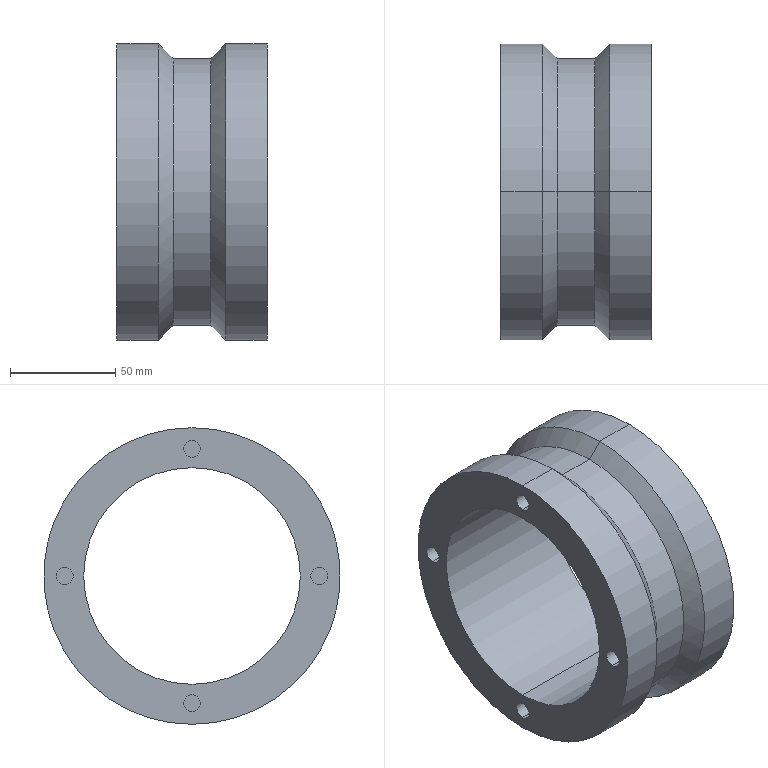Part | SolidWorks | features ICE 2, Revolution 1 | 1 solid | 38 faces | box 71.5 x 141 x 141 mm | volume 441421 mm3 | cylinder 24 | plane 10 | cone 4 | commonest cylinder face diameters 8 x16 141 x4 103 x2 127 x2
STEP:
#1=CARTESIAN_POINT('',(21.275,0.,64.5));
#2=VERTEX_POINT('',#1);
#3=CARTESIAN_POINT('',(21.275,0.,56.5));
#4=VERTEX_POINT('',#3);
#5=CARTESIAN_POINT('',(21.275,0.,60.5));
#6=DIRECTION('',(1.,0.,0.));
#7=DIRECTION('',(0.,0.,-1.));
#8=AXIS2_PLACEMENT_3D('',#5,#6,#7);
#9=CIRCLE('',#8,4.);
#10=EDGE_CURVE('',#2,#4,#9,.T.);
#11=ORIENTED_EDGE('',*,*,#10,.F.);
#12=CARTESIAN_POINT('',(34.275,0.,64.5));
#13=VERTEX_POINT('',#12);
#14=CARTESIAN_POINT('',(21.275,0.,64.5));
#15=DIRECTION('',(1.,0.,0.));
#16=VECTOR('',#15,1000.);
#17=LINE('',#14,#16);
#18=EDGE_CURVE('',#2,#13,#17,.T.);
#19=ORIENTED_EDGE('',*,*,#18,.T.);
#20=CARTESIAN_POINT('',(34.275,0.,56.5));
#21=VERTEX_POINT('',#20);
#22=CARTESIAN_POINT('',(34.275,0.,60.5));
#23=DIRECTION('',(1.,0.,0.));
#24=DIRECTION('',(0.,0.,-1.));
#25=AXIS2_PLACEMENT_3D('',#22,#23,#24);
#26=CIRCLE('',#25,4.);
#27=EDGE_CURVE('',#13,#21,#26,.T.);
#28=ORIENTED_EDGE('',*,*,#27,.T.);
#29=CARTESIAN_POINT('',(21.275,0.,56.5));
#30=DIRECTION('',(1.,0.,0.));
#31=VECTOR('',#30,1000.);
#32=LINE('',#29,#31);
#33=EDGE_CURVE('',#4,#21,#32,.T.);
#34=ORIENTED_EDGE('',*,*,#33,.F.);
#35=EDGE_LOOP('',(#11,#19,#28,#34));
#36=FACE_OUTER_BOUND('',#35,.T.);
#37=CARTESIAN_POINT('',(21.275,0.,60.5));
#38=DIRECTION('',(1.,0.,0.));
#39=DIRECTION('',(0.,0.,-1.));
#40=AXIS2_PLACEMENT_3D('',#37,#38,#39);
#41=CYLINDRICAL_SURFACE('',#40,4.);
#42=ADVANCED_FACE('',(#36),#41,.F.);
#43=CARTESIAN_POINT('',(21.275,60.5,4.));
#44=VERTEX_POINT('',#43);
#45=CARTESIAN_POINT('',(21.275,60.5,-4.));
#46=VERTEX_POINT('',#45);
#47=CARTESIAN_POINT('',(21.275,60.5,0.));
#48=DIRECTION('',(1.,0.,0.));
#49=DIRECTION('',(0.,0.,-1.));
#50=AXIS2_PLACEMENT_3D('',#47,#48,#49);
#51=CIRCLE('',#50,4.);
#52=EDGE_CURVE('',#44,#46,#51,.T.);
#53=ORIENTED_EDGE('',*,*,#52,.F.);
#54=CARTESIAN_POINT('',(34.275,60.5,4.));
#55=VERTEX_POINT('',#54);
#56=CARTESIAN_POINT('',(21.275,60.5,4.));
#57=DIRECTION('',(1.,0.,0.));
#58=VECTOR('',#57,1000.);
#59=LINE('',#56,#58);
#60=EDGE_CURVE('',#44,#55,#59,.T.);
#61=ORIENTED_EDGE('',*,*,#60,.T.);
#62=CARTESIAN_POINT('',(34.275,60.5,-4.));
#63=VERTEX_POINT('',#62);
#64=CARTESIAN_POINT('',(34.275,60.5,0.));
#65=DIRECTION('',(1.,0.,0.));
#66=DIRECTION('',(0.,0.,-1.));
#67=AXIS2_PLACEMENT_3D('',#64,#65,#66);
#68=CIRCLE('',#67,4.);
#69=EDGE_CURVE('',#55,#63,#68,.T.);
#70=ORIENTED_EDGE('',*,*,#69,.T.);
#71=CARTESIAN_POINT('',(21.275,60.5,-4.));
#72=DIRECTION('',(1.,0.,0.));
#73=VECTOR('',#72,1000.);
#74=LINE('',#71,#73);
#75=EDGE_CURVE('',#46,#63,#74,.T.);
#76=ORIENTED_EDGE('',*,*,#75,.F.);
#77=EDGE_LOOP('',(#53,#61,#70,#76));
#78=FACE_OUTER_BOUND('',#77,.T.);
#79=CARTESIAN_POINT('',(21.275,60.5,0.));
#80=DIRECTION('',(1.,0.,0.));
#81=DIRECTION('',(0.,0.,-1.));
#82=AXIS2_PLACEMENT_3D('',#79,#80,#81);
#83=CYLINDRICAL_SURFACE('',#82,4.);
#84=ADVANCED_FACE('',(#78),#83,.F.);
#85=CARTESIAN_POINT('',(21.275,0.,-56.5));
#86=VERTEX_POINT('',#85);
#87=CARTESIAN_POINT('',(21.275,0.,-64.5));
#88=VERTEX_POINT('',#87);
#89=CARTESIAN_POINT('',(21.275,0.,-60.5));
#90=DIRECTION('',(1.,0.,0.));
#91=DIRECTION('',(0.,0.,-1.));
#92=AXIS2_PLACEMENT_3D('',#89,#90,#91);
#93=CIRCLE('',#92,4.);
#94=EDGE_CURVE('',#86,#88,#93,.T.);
#95=ORIENTED_EDGE('',*,*,#94,.F.);
#96=CARTESIAN_POINT('',(34.275,0.,-56.5));
#97=VERTEX_POINT('',#96);
#98=CARTESIAN_POINT('',(21.275,0.,-56.5));
#99=DIRECTION('',(1.,0.,0.));
#100=VECTOR('',#99,1000.);
#101=LINE('',#98,#100);
#102=EDGE_CURVE('',#86,#97,#101,.T.);
#103=ORIENTED_EDGE('',*,*,#102,.T.);
#104=CARTESIAN_POINT('',(34.275,0.,-64.5));
#105=VERTEX_POINT('',#104);
#106=CARTESIAN_POINT('',(34.275,0.,-60.5));
#107=DIRECTION('',(1.,0.,0.));
#108=DIRECTION('',(0.,0.,-1.));
#109=AXIS2_PLACEMENT_3D('',#106,#107,#108);
#110=CIRCLE('',#109,4.);
#111=EDGE_CURVE('',#97,#105,#110,.T.);
#112=ORIENTED_EDGE('',*,*,#111,.T.);
#113=CARTESIAN_POINT('',(21.275,0.,-64.5));
#114=DIRECTION('',(1.,0.,0.));
#115=VECTOR('',#114,1000.);
#116=LINE('',#113,#115);
#117=EDGE_CURVE('',#88,#105,#116,.T.);
#118=ORIENTED_EDGE('',*,*,#117,.F.);
#119=EDGE_LOOP('',(#95,#103,#112,#118));
#120=FACE_OUTER_BOUND('',#119,.T.);
#121=CARTESIAN_POINT('',(21.275,0.,-60.5));
#122=DIRECTION('',(1.,0.,0.));
#123=DIRECTION('',(0.,0.,-1.));
#124=AXIS2_PLACEMENT_3D('',#121,#122,#123);
#125=CYLINDRICAL_SURFACE('',#124,4.);
#126=ADVANCED_FACE('',(#120),#125,.F.);
#127=CARTESIAN_POINT('',(21.275,-60.5,4.));
#128=VERTEX_POINT('',#127);
#129=CARTESIAN_POINT('',(21.275,-60.5,-4.));
#130=VERTEX_POINT('',#129);
#131=CARTESIAN_POINT('',(21.275,-60.5,0.));
#132=DIRECTION('',(1.,0.,0.));
#133=DIRECTION('',(0.,0.,-1.));
#134=AXIS2_PLACEMENT_3D('',#131,#132,#133);
#135=CIRCLE('',#134,4.);
#136=EDGE_CURVE('',#128,#130,#135,.T.);
#137=ORIENTED_EDGE('',*,*,#136,.F.);
#138=CARTESIAN_POINT('',(34.275,-60.5,4.));
#139=VERTEX_POINT('',#138);
#140=CARTESIAN_POINT('',(21.275,-60.5,4.));
#141=DIRECTION('',(1.,0.,0.));
#142=VECTOR('',#141,1000.);
#143=LINE('',#140,#142);
#144=EDGE_CURVE('',#128,#139,#143,.T.);
#145=ORIENTED_EDGE('',*,*,#144,.T.);
#146=CARTESIAN_POINT('',(34.275,-60.5,-4.));
#147=VERTEX_POINT('',#146);
#148=CARTESIAN_POINT('',(34.275,-60.5,0.));
#149=DIRECTION('',(1.,0.,0.));
#150=DIRECTION('',(0.,0.,-1.));
#151=AXIS2_PLACEMENT_3D('',#148,#149,#150);
#152=CIRCLE('',#151,4.);
#153=EDGE_CURVE('',#139,#147,#152,.T.);
#154=ORIENTED_EDGE('',*,*,#153,.T.);
#155=CARTESIAN_POINT('',(21.275,-60.5,-4.));
#156=DIRECTION('',(1.,0.,0.));
#157=VECTOR('',#156,1000.);
#158=LINE('',#155,#157);
#159=EDGE_CURVE('',#130,#147,#158,.T.);
#160=ORIENTED_EDGE('',*,*,#159,.F.);
#161=EDGE_LOOP('',(#137,#145,#154,#160));
#162=FACE_OUTER_BOUND('',#161,.T.);
#163=CARTESIAN_POINT('',(21.275,-60.5,0.));
#164=DIRECTION('',(1.,0.,0.));
#165=DIRECTION('',(0.,0.,-1.));
#166=AXIS2_PLACEMENT_3D('',#163,#164,#165);
#167=CYLINDRICAL_SURFACE('',#166,4.);
#168=ADVANCED_FACE('',(#162),#167,.F.);
#169=CARTESIAN_POINT('',(-24.225,0.,-64.5));
#170=VERTEX_POINT('',#169);
#171=CARTESIAN_POINT('',(-24.225,0.,-56.5));
#172=VERTEX_POINT('',#171);
#173=CARTESIAN_POINT('',(-24.225,0.,-60.5));
#174=DIRECTION('',(-1.,0.,0.));
#175=DIRECTION('',(0.,0.,1.));
#176=AXIS2_PLACEMENT_3D('',#173,#174,#175);
#177=CIRCLE('',#176,4.);
#178=EDGE_CURVE('',#170,#172,#177,.T.);
#179=ORIENTED_EDGE('',*,*,#178,.F.);
#180=CARTESIAN_POINT('',(-37.225,0.,-64.5));
#181=VERTEX_POINT('',#180);
#182=CARTESIAN_POINT('',(-24.225,0.,-64.5));
#183=DIRECTION('',(-1.,0.,0.));
#184=VECTOR('',#183,1000.);
#185=LINE('',#182,#184);
#186=EDGE_CURVE('',#170,#181,#185,.T.);
#187=ORIENTED_EDGE('',*,*,#186,.T.);
#188=CARTESIAN_POINT('',(-37.225,0.,-56.5));
#189=VERTEX_POINT('',#188);
#190=CARTESIAN_POINT('',(-37.225,0.,-60.5));
#191=DIRECTION('',(-1.,0.,0.));
#192=DIRECTION('',(0.,0.,1.));
#193=AXIS2_PLACEMENT_3D('',#190,#191,#192);
#194=CIRCLE('',#193,4.);
#195=EDGE_CURVE('',#181,#189,#194,.T.);
#196=ORIENTED_EDGE('',*,*,#195,.T.);
#197=CARTESIAN_POINT('',(-24.225,0.,-56.5));
#198=DIRECTION('',(-1.,0.,0.));
#199=VECTOR('',#198,1000.);
#200=LINE('',#197,#199);
#201=EDGE_CURVE('',#172,#189,#200,.T.);
#202=ORIENTED_EDGE('',*,*,#201,.F.);
#203=EDGE_LOOP('',(#179,#187,#196,#202));
#204=FACE_OUTER_BOUND('',#203,.T.);
#205=CARTESIAN_POINT('',(-24.225,0.,-60.5));
#206=DIRECTION('',(-1.,0.,0.));
#207=DIRECTION('',(0.,0.,1.));
#208=AXIS2_PLACEMENT_3D('',#205,#206,#207);
#209=CYLINDRICAL_SURFACE('',#208,4.);
#210=ADVANCED_FACE('',(#204),#209,.F.);
#211=CARTESIAN_POINT('',(-24.225,60.5,-4.));
#212=VERTEX_POINT('',#211);
#213=CARTESIAN_POINT('',(-24.225,60.5,4.));
#214=VERTEX_POINT('',#213);
#215=CARTESIAN_POINT('',(-24.225,60.5,0.));
#216=DIRECTION('',(-1.,0.,0.));
#217=DIRECTION('',(0.,0.,1.));
#218=AXIS2_PLACEMENT_3D('',#215,#216,#217);
#219=CIRCLE('',#218,4.);
#220=EDGE_CURVE('',#212,#214,#219,.T.);
#221=ORIENTED_EDGE('',*,*,#220,.F.);
#222=CARTESIAN_POINT('',(-37.225,60.5,-4.));
#223=VERTEX_POINT('',#222);
#224=CARTESIAN_POINT('',(-24.225,60.5,-4.));
#225=DIRECTION('',(-1.,0.,0.));
#226=VECTOR('',#225,1000.);
#227=LINE('',#224,#226);
#228=EDGE_CURVE('',#212,#223,#227,.T.);
#229=ORIENTED_EDGE('',*,*,#228,.T.);
#230=CARTESIAN_POINT('',(-37.225,60.5,4.));
#231=VERTEX_POINT('',#230);
#232=CARTESIAN_POINT('',(-37.225,60.5,0.));
#233=DIRECTION('',(-1.,0.,0.));
#234=DIRECTION('',(0.,0.,1.));
#235=AXIS2_PLACEMENT_3D('',#232,#233,#234);
#236=CIRCLE('',#235,4.);
#237=EDGE_CURVE('',#223,#231,#236,.T.);
#238=ORIENTED_EDGE('',*,*,#237,.T.);
#239=CARTESIAN_POINT('',(-24.225,60.5,4.));
#240=DIRECTION('',(-1.,0.,0.));
#241=VECTOR('',#240,1000.);
#242=LINE('',#239,#241);
#243=EDGE_CURVE('',#214,#231,#242,.T.);
#244=ORIENTED_EDGE('',*,*,#243,.F.);
#245=EDGE_LOOP('',(#221,#229,#238,#244));
#246=FACE_OUTER_BOUND('',#245,.T.);
#247=CARTESIAN_POINT('',(-24.225,60.5,0.));
#248=DIRECTION('',(-1.,0.,0.));
#249=DIRECTION('',(0.,0.,1.));
#250=AXIS2_PLACEMENT_3D('',#247,#248,#249);
#251=CYLINDRICAL_SURFACE('',#250,4.);
#252=ADVANCED_FACE('',(#246),#251,.F.);
#253=CARTESIAN_POINT('',(-24.225,0.,56.5));
#254=VERTEX_POINT('',#253);
#255=CARTESIAN_POINT('',(-24.225,0.,64.5));
#256=VERTEX_POINT('',#255);
#257=CARTESIAN_POINT('',(-24.225,0.,60.5));
#258=DIRECTION('',(-1.,0.,0.));
#259=DIRECTION('',(0.,0.,1.));
#260=AXIS2_PLACEMENT_3D('',#257,#258,#259);
#261=CIRCLE('',#260,4.);
#262=EDGE_CURVE('',#254,#256,#261,.T.);
#263=ORIENTED_EDGE('',*,*,#262,.F.);
#264=CARTESIAN_POINT('',(-37.225,0.,56.5));
#265=VERTEX_POINT('',#264);
#266=CARTESIAN_POINT('',(-24.225,0.,56.5));
#267=DIRECTION('',(-1.,0.,0.));
#268=VECTOR('',#267,1000.);
#269=LINE('',#266,#268);
#270=EDGE_CURVE('',#254,#265,#269,.T.);
#271=ORIENTED_EDGE('',*,*,#270,.T.);
#272=CARTESIAN_POINT('',(-37.225,0.,64.5));
#273=VERTEX_POINT('',#272);
#274=CARTESIAN_POINT('',(-37.225,0.,60.5));
#275=DIRECTION('',(-1.,0.,0.));
#276=DIRECTION('',(0.,0.,1.));
#277=AXIS2_PLACEMENT_3D('',#274,#275,#276);
#278=CIRCLE('',#277,4.);
#279=EDGE_CURVE('',#265,#273,#278,.T.);
#280=ORIENTED_EDGE('',*,*,#279,.T.);
#281=CARTESIAN_POINT('',(-24.225,0.,64.5));
#282=DIRECTION('',(-1.,0.,0.));
#283=VECTOR('',#282,1000.);
#284=LINE('',#281,#283);
#285=EDGE_CURVE('',#256,#273,#284,.T.);
#286=ORIENTED_EDGE('',*,*,#285,.F.);
#287=EDGE_LOOP('',(#263,#271,#280,#286));
#288=FACE_OUTER_BOUND('',#287,.T.);
#289=CARTESIAN_POINT('',(-24.225,0.,60.5));
#290=DIRECTION('',(-1.,0.,0.));
#291=DIRECTION('',(0.,0.,1.));
#292=AXIS2_PLACEMENT_3D('',#289,#290,#291);
#293=CYLINDRICAL_SURFACE('',#292,4.);
#294=ADVANCED_FACE('',(#288),#293,.F.);
#295=CARTESIAN_POINT('',(-24.225,-60.5,-4.));
#296=VERTEX_POINT('',#295);
#297=CARTESIAN_POINT('',(-24.225,-60.5,4.));
#298=VERTEX_POINT('',#297);
#299=CARTESIAN_POINT('',(-24.225,-60.5,0.));
#300=DIRECTION('',(-1.,0.,0.));
#301=DIRECTION('',(0.,0.,1.));
#302=AXIS2_PLACEMENT_3D('',#299,#300,#301);
#303=CIRCLE('',#302,4.);
#304=EDGE_CURVE('',#296,#298,#303,.T.);
#305=ORIENTED_EDGE('',*,*,#304,.F.);
#306=CARTESIAN_POINT('',(-37.225,-60.5,-4.));
#307=VERTEX_POINT('',#306);
#308=CARTESIAN_POINT('',(-24.225,-60.5,-4.));
#309=DIRECTION('',(-1.,0.,0.));
#310=VECTOR('',#309,1000.);
#311=LINE('',#308,#310);
#312=EDGE_CURVE('',#296,#307,#311,.T.);
#313=ORIENTED_EDGE('',*,*,#312,.T.);
#314=CARTESIAN_POINT('',(-37.225,-60.5,4.));
#315=VERTEX_POINT('',#314);
#316=CARTESIAN_POINT('',(-37.225,-60.5,0.));
#317=DIRECTION('',(-1.,0.,0.));
#318=DIRECTION('',(0.,0.,1.));
#319=AXIS2_PLACEMENT_3D('',#316,#317,#318);
#320=CIRCLE('',#319,4.);
#321=EDGE_CURVE('',#307,#315,#320,.T.);
#322=ORIENTED_EDGE('',*,*,#321,.T.);
#323=CARTESIAN_POINT('',(-24.225,-60.5,4.));
#324=DIRECTION('',(-1.,0.,0.));
#325=VECTOR('',#324,1000.);
#326=LINE('',#323,#325);
#327=EDGE_CURVE('',#298,#315,#326,.T.);
#328=ORIENTED_EDGE('',*,*,#327,.F.);
#329=EDGE_LOOP('',(#305,#313,#322,#328));
#330=FACE_OUTER_BOUND('',#329,.T.);
#331=CARTESIAN_POINT('',(-24.225,-60.5,0.));
#332=DIRECTION('',(-1.,0.,0.));
#333=DIRECTION('',(0.,0.,1.));
#334=AXIS2_PLACEMENT_3D('',#331,#332,#333);
#335=CYLINDRICAL_SURFACE('',#334,4.);
#336=ADVANCED_FACE('',(#330),#335,.F.);
#337=CARTESIAN_POINT('',(-10.475,0.,63.5));
#338=VERTEX_POINT('',#337);
#339=CARTESIAN_POINT('',(-10.475,0.,-63.5));
#340=VERTEX_POINT('',#339);
#341=CARTESIAN_POINT('',(-10.475,0.,0.));
#342=DIRECTION('',(-1.,0.,0.));
#343=DIRECTION('',(0.,0.,1.));
#344=AXIS2_PLACEMENT_3D('',#341,#342,#343);
#345=CIRCLE('',#344,63.5);
#346=EDGE_CURVE('',#338,#340,#345,.T.);
#347=ORIENTED_EDGE('',*,*,#346,.T.);
#348=CARTESIAN_POINT('',(-17.475,0.,-70.5));
#349=VERTEX_POINT('',#348);
#350=CARTESIAN_POINT('',(-10.475,0.,-63.5));
#351=DIRECTION('',(-0.7071,0.,-0.7071));
#352=VECTOR('',#351,1000.);
#353=LINE('',#350,#352);
#354=EDGE_CURVE('',#340,#349,#353,.T.);
#355=ORIENTED_EDGE('',*,*,#354,.T.);
#356=CARTESIAN_POINT('',(-17.475,0.,70.5));
#357=VERTEX_POINT('',#356);
#358=CARTESIAN_POINT('',(-17.475,0.,0.));
#359=DIRECTION('',(-1.,0.,0.));
#360=DIRECTION('',(0.,0.,1.));
#361=AXIS2_PLACEMENT_3D('',#358,#359,#360);
#362=CIRCLE('',#361,70.5);
#363=EDGE_CURVE('',#357,#349,#362,.T.);
#364=ORIENTED_EDGE('',*,*,#363,.F.);
#365=CARTESIAN_POINT('',(-10.475,0.,63.5));
#366=DIRECTION('',(-0.7071,0.,0.7071));
#367=VECTOR('',#366,1000.);
#368=LINE('',#365,#367);
#369=EDGE_CURVE('',#338,#357,#368,.T.);
#370=ORIENTED_EDGE('',*,*,#369,.F.);
#371=EDGE_LOOP('',(#347,#355,#364,#370));
#372=FACE_OUTER_BOUND('',#371,.T.);
#373=CARTESIAN_POINT('',(-10.475,0.,0.));
#374=DIRECTION('',(-1.,0.,0.));
#375=DIRECTION('',(0.,0.,1.));
#376=AXIS2_PLACEMENT_3D('',#373,#374,#375);
#377=CONICAL_SURFACE('',#376,63.5,0.7854);
#378=ADVANCED_FACE('',(#372),#377,.T.);
#379=CARTESIAN_POINT('',(7.525,0.,63.5));
#380=VERTEX_POINT('',#379);
#381=CARTESIAN_POINT('',(7.525,0.,-63.5));
#382=VERTEX_POINT('',#381);
#383=CARTESIAN_POINT('',(7.525,0.,0.));
#384=DIRECTION('',(-1.,0.,0.));
#385=DIRECTION('',(0.,0.,1.));
#386=AXIS2_PLACEMENT_3D('',#383,#384,#385);
#387=CIRCLE('',#386,63.5);
#388=EDGE_CURVE('',#380,#382,#387,.T.);
#389=ORIENTED_EDGE('',*,*,#388,.T.);
#390=CARTESIAN_POINT('',(-86.708,0.,-63.5));
#391=DIRECTION('',(-1.,0.,0.));
#392=VECTOR('',#391,1000.);
#393=LINE('',#390,#392);
#394=EDGE_CURVE('',#382,#340,#393,.T.);
#395=ORIENTED_EDGE('',*,*,#394,.T.);
#396=ORIENTED_EDGE('',*,*,#346,.F.);
#397=CARTESIAN_POINT('',(-86.708,0.,63.5));
#398=DIRECTION('',(-1.,0.,0.));
#399=VECTOR('',#398,1000.);
#400=LINE('',#397,#399);
#401=EDGE_CURVE('',#380,#338,#400,.T.);
#402=ORIENTED_EDGE('',*,*,#401,.F.);
#403=EDGE_LOOP('',(#389,#395,#396,#402));
#404=FACE_OUTER_BOUND('',#403,.T.);
#405=CARTESIAN_POINT('',(-86.708,0.,0.));
#406=DIRECTION('',(-1.,0.,0.));
#407=DIRECTION('',(0.,0.,1.));
#408=AXIS2_PLACEMENT_3D('',#405,#406,#407);
#409=CYLINDRICAL_SURFACE('',#408,63.5);
#410=ADVANCED_FACE('',(#404),#409,.T.);
#411=ORIENTED_EDGE('',*,*,#388,.F.);
#412=CARTESIAN_POINT('',(14.525,0.,70.5));
#413=VERTEX_POINT('',#412);
#414=CARTESIAN_POINT('',(14.525,0.,70.5));
#415=DIRECTION('',(0.7071,0.,0.7071));
#416=VECTOR('',#415,1000.);
#417=LINE('',#414,#416);
#418=EDGE_CURVE('',#380,#413,#417,.T.);
#419=ORIENTED_EDGE('',*,*,#418,.T.);
#420=CARTESIAN_POINT('',(14.525,0.,-70.5));
#421=VERTEX_POINT('',#420);
#422=CARTESIAN_POINT('',(14.525,0.,0.));
#423=DIRECTION('',(-1.,0.,0.));
#424=DIRECTION('',(0.,0.,1.));
#425=AXIS2_PLACEMENT_3D('',#422,#423,#424);
#426=CIRCLE('',#425,70.5);
#427=EDGE_CURVE('',#413,#421,#426,.T.);
#428=ORIENTED_EDGE('',*,*,#427,.T.);
#429=CARTESIAN_POINT('',(14.525,0.,-70.5));
#430=DIRECTION('',(0.7071,0.,-0.7071));
#431=VECTOR('',#430,1000.);
#432=LINE('',#429,#431);
#433=EDGE_CURVE('',#382,#421,#432,.T.);
#434=ORIENTED_EDGE('',*,*,#433,.F.);
#435=EDGE_LOOP('',(#411,#419,#428,#434));
#436=FACE_OUTER_BOUND('',#435,.T.);
#437=CARTESIAN_POINT('',(14.525,0.,0.));
#438=DIRECTION('',(1.,0.,0.));
#439=DIRECTION('',(0.,0.,-1.));
#440=AXIS2_PLACEMENT_3D('',#437,#438,#439);
#441=CONICAL_SURFACE('',#440,70.5,0.7854);
#442=ADVANCED_FACE('',(#436),#441,.T.);
#443=CARTESIAN_POINT('',(34.275,0.,70.5));
#444=VERTEX_POINT('',#443);
#445=CARTESIAN_POINT('',(34.275,0.,-70.5));
#446=VERTEX_POINT('',#445);
#447=CARTESIAN_POINT('',(34.275,0.,0.));
#448=DIRECTION('',(-1.,0.,0.));
#449=DIRECTION('',(0.,0.,1.));
#450=AXIS2_PLACEMENT_3D('',#447,#448,#449);
#451=CIRCLE('',#450,70.5);
#452=EDGE_CURVE('',#444,#446,#451,.T.);
#453=ORIENTED_EDGE('',*,*,#452,.T.);
#454=CARTESIAN_POINT('',(-86.708,0.,-70.5));
#455=DIRECTION('',(-1.,0.,0.));
#456=VECTOR('',#455,1000.);
#457=LINE('',#454,#456);
#458=EDGE_CURVE('',#446,#421,#457,.T.);
#459=ORIENTED_EDGE('',*,*,#458,.T.);
#460=ORIENTED_EDGE('',*,*,#427,.F.);
#461=CARTESIAN_POINT('',(-86.708,0.,70.5));
#462=DIRECTION('',(-1.,0.,0.));
#463=VECTOR('',#462,1000.);
#464=LINE('',#461,#463);
#465=EDGE_CURVE('',#444,#413,#464,.T.);
#466=ORIENTED_EDGE('',*,*,#465,.F.);
#467=EDGE_LOOP('',(#453,#459,#460,#466));
#468=FACE_OUTER_BOUND('',#467,.T.);
#469=CARTESIAN_POINT('',(-86.708,0.,0.));
#470=DIRECTION('',(-1.,0.,0.));
#471=DIRECTION('',(0.,0.,1.));
#472=AXIS2_PLACEMENT_3D('',#469,#470,#471);
#473=CYLINDRICAL_SURFACE('',#472,70.5);
#474=ADVANCED_FACE('',(#468),#473,.T.);
#475=CARTESIAN_POINT('',(34.275,0.,-51.5));
#476=VERTEX_POINT('',#475);
#477=CARTESIAN_POINT('',(34.275,0.,51.5));
#478=VERTEX_POINT('',#477);
#479=CARTESIAN_POINT('',(34.275,0.,0.));
#480=DIRECTION('',(-1.,0.,0.));
#481=DIRECTION('',(0.,0.,1.));
#482=AXIS2_PLACEMENT_3D('',#479,#480,#481);
#483=CIRCLE('',#482,51.5);
#484=EDGE_CURVE('',#476,#478,#483,.T.);
#485=ORIENTED_EDGE('',*,*,#484,.F.);
#486=CARTESIAN_POINT('',(-37.225,0.,-51.5));
#487=VERTEX_POINT('',#486);
#488=CARTESIAN_POINT('',(-86.708,0.,-51.5));
#489=DIRECTION('',(-1.,0.,0.));
#490=VECTOR('',#489,1000.);
#491=LINE('',#488,#490);
#492=EDGE_CURVE('',#476,#487,#491,.T.);
#493=ORIENTED_EDGE('',*,*,#492,.T.);
#494=CARTESIAN_POINT('',(-37.225,0.,51.5));
#495=VERTEX_POINT('',#494);
#496=CARTESIAN_POINT('',(-37.225,0.,0.));
#497=DIRECTION('',(-1.,0.,0.));
#498=DIRECTION('',(0.,0.,1.));
#499=AXIS2_PLACEMENT_3D('',#496,#497,#498);
#500=CIRCLE('',#499,51.5);
#501=EDGE_CURVE('',#487,#495,#500,.T.);
#502=ORIENTED_EDGE('',*,*,#501,.T.);
#503=CARTESIAN_POINT('',(-86.708,0.,51.5));
#504=DIRECTION('',(-1.,0.,0.));
#505=VECTOR('',#504,1000.);
#506=LINE('',#503,#505);
#507=EDGE_CURVE('',#478,#495,#506,.T.);
#508=ORIENTED_EDGE('',*,*,#507,.F.);
#509=EDGE_LOOP('',(#485,#493,#502,#508));
#510=FACE_OUTER_BOUND('',#509,.T.);
#511=CARTESIAN_POINT('',(-86.708,0.,0.));
#512=DIRECTION('',(-1.,0.,0.));
#513=DIRECTION('',(0.,0.,1.));
#514=AXIS2_PLACEMENT_3D('',#511,#512,#513);
#515=CYLINDRICAL_SURFACE('',#514,51.5);
#516=ADVANCED_FACE('',(#510),#515,.F.);
#517=ORIENTED_EDGE('',*,*,#363,.T.);
#518=CARTESIAN_POINT('',(-37.225,0.,-70.5));
#519=VERTEX_POINT('',#518);
#520=CARTESIAN_POINT('',(-86.708,0.,-70.5));
#521=DIRECTION('',(-1.,0.,0.));
#522=VECTOR('',#521,1000.);
#523=LINE('',#520,#522);
#524=EDGE_CURVE('',#349,#519,#523,.T.);
#525=ORIENTED_EDGE('',*,*,#524,.T.);
#526=CARTESIAN_POINT('',(-37.225,0.,70.5));
#527=VERTEX_POINT('',#526);
#528=CARTESIAN_POINT('',(-37.225,0.,0.));
#529=DIRECTION('',(-1.,0.,0.));
#530=DIRECTION('',(0.,0.,1.));
#531=AXIS2_PLACEMENT_3D('',#528,#529,#530);
#532=CIRCLE('',#531,70.5);
#533=EDGE_CURVE('',#527,#519,#532,.T.);
#534=ORIENTED_EDGE('',*,*,#533,.F.);
#535=CARTESIAN_POINT('',(-86.708,0.,70.5));
#536=DIRECTION('',(-1.,0.,0.));
#537=VECTOR('',#536,1000.);
#538=LINE('',#535,#537);
#539=EDGE_CURVE('',#357,#527,#538,.T.);
#540=ORIENTED_EDGE('',*,*,#539,.F.);
#541=EDGE_LOOP('',(#517,#525,#534,#540));
#542=FACE_OUTER_BOUND('',#541,.T.);
#543=CARTESIAN_POINT('',(-86.708,0.,0.));
#544=DIRECTION('',(-1.,0.,0.));
#545=DIRECTION('',(0.,0.,1.));
#546=AXIS2_PLACEMENT_3D('',#543,#544,#545);
#547=CYLINDRICAL_SURFACE('',#546,70.5);
#548=ADVANCED_FACE('',(#542),#547,.T.);
#549=ORIENTED_EDGE('',*,*,#524,.F.);
#550=CARTESIAN_POINT('',(-17.475,0.,0.));
#551=DIRECTION('',(-1.,0.,0.));
#552=DIRECTION('',(0.,0.,1.));
#553=AXIS2_PLACEMENT_3D('',#550,#551,#552);
#554=CIRCLE('',#553,70.5);
#555=EDGE_CURVE('',#349,#357,#554,.T.);
#556=ORIENTED_EDGE('',*,*,#555,.T.);
#557=ORIENTED_EDGE('',*,*,#539,.T.);
#558=CARTESIAN_POINT('',(-37.225,0.,0.));
#559=DIRECTION('',(-1.,0.,0.));
#560=DIRECTION('',(0.,0.,1.));
#561=AXIS2_PLACEMENT_3D('',#558,#559,#560);
#562=CIRCLE('',#561,70.5);
#563=EDGE_CURVE('',#519,#527,#562,.T.);
#564=ORIENTED_EDGE('',*,*,#563,.F.);
#565=EDGE_LOOP('',(#549,#556,#557,#564));
#566=FACE_OUTER_BOUND('',#565,.T.);
#567=CARTESIAN_POINT('',(-86.708,0.,0.));
#568=DIRECTION('',(-1.,0.,0.));
#569=DIRECTION('',(0.,0.,1.));
#570=AXIS2_PLACEMENT_3D('',#567,#568,#569);
#571=CYLINDRICAL_SURFACE('',#570,70.5);
#572=ADVANCED_FACE('',(#566),#571,.T.);
#573=CARTESIAN_POINT('',(-37.225,0.,-60.5));
#574=DIRECTION('',(-1.,0.,0.));
#575=DIRECTION('',(0.,0.,1.));
#576=AXIS2_PLACEMENT_3D('',#573,#574,#575);
#577=CIRCLE('',#576,4.);
#578=EDGE_CURVE('',#189,#181,#577,.T.);
#579=ORIENTED_EDGE('',*,*,#578,.F.);
#580=ORIENTED_EDGE('',*,*,#195,.F.);
#581=EDGE_LOOP('',(#579,#580));
#582=FACE_BOUND('',#581,.T.);
#583=CARTESIAN_POINT('',(-37.225,60.5,0.));
#584=DIRECTION('',(-1.,0.,0.));
#585=DIRECTION('',(0.,0.,1.));
#586=AXIS2_PLACEMENT_3D('',#583,#584,#585);
#587=CIRCLE('',#586,4.);
#588=EDGE_CURVE('',#231,#223,#587,.T.);
#589=ORIENTED_EDGE('',*,*,#588,.F.);
#590=ORIENTED_EDGE('',*,*,#237,.F.);
#591=EDGE_LOOP('',(#589,#590));
#592=FACE_BOUND('',#591,.T.);
#593=CARTESIAN_POINT('',(-37.225,0.,60.5));
#594=DIRECTION('',(-1.,0.,0.));
#595=DIRECTION('',(0.,0.,1.));
#596=AXIS2_PLACEMENT_3D('',#593,#594,#595);
#597=CIRCLE('',#596,4.);
#598=EDGE_CURVE('',#273,#265,#597,.T.);
#599=ORIENTED_EDGE('',*,*,#598,.F.);
#600=ORIENTED_EDGE('',*,*,#279,.F.);
#601=EDGE_LOOP('',(#599,#600));
#602=FACE_BOUND('',#601,.T.);
#603=CARTESIAN_POINT('',(-37.225,-60.5,0.));
#604=DIRECTION('',(-1.,0.,0.));
#605=DIRECTION('',(0.,0.,1.));
#606=AXIS2_PLACEMENT_3D('',#603,#604,#605);
#607=CIRCLE('',#606,4.);
#608=EDGE_CURVE('',#315,#307,#607,.T.);
#609=ORIENTED_EDGE('',*,*,#608,.F.);
#610=ORIENTED_EDGE('',*,*,#321,.F.);
#611=EDGE_LOOP('',(#609,#610));
#612=FACE_BOUND('',#611,.T.);
#613=CARTESIAN_POINT('',(-37.225,0.,0.));
#614=DIRECTION('',(-1.,0.,0.));
#615=DIRECTION('',(0.,0.,1.));
#616=AXIS2_PLACEMENT_3D('',#613,#614,#615);
#617=CIRCLE('',#616,51.5);
#618=EDGE_CURVE('',#495,#487,#617,.T.);
#619=ORIENTED_EDGE('',*,*,#618,.F.);
#620=ORIENTED_EDGE('',*,*,#501,.F.);
#621=EDGE_LOOP('',(#619,#620));
#622=FACE_BOUND('',#621,.T.);
#623=ORIENTED_EDGE('',*,*,#533,.T.);
#624=ORIENTED_EDGE('',*,*,#563,.T.);
#625=EDGE_LOOP('',(#623,#624));
#626=FACE_OUTER_BOUND('',#625,.T.);
#627=CARTESIAN_POINT('',(-37.225,70.5,0.));
#628=DIRECTION('',(1.,0.,0.));
#629=DIRECTION('',(0.,0.,-1.));
#630=AXIS2_PLACEMENT_3D('',#627,#628,#629);
#631=PLANE('',#630);
#632=ADVANCED_FACE('',(#582,#592,#602,#612,#622,#626),#631,.F.);
#633=ORIENTED_EDGE('',*,*,#492,.F.);
#634=CARTESIAN_POINT('',(34.275,0.,0.));
#635=DIRECTION('',(-1.,0.,0.));
#636=DIRECTION('',(0.,0.,1.));
#637=AXIS2_PLACEMENT_3D('',#634,#635,#636);
#638=CIRCLE('',#637,51.5);
#639=EDGE_CURVE('',#478,#476,#638,.T.);
#640=ORIENTED_EDGE('',*,*,#639,.F.);
#641=ORIENTED_EDGE('',*,*,#507,.T.);
#642=ORIENTED_EDGE('',*,*,#618,.T.);
#643=EDGE_LOOP('',(#633,#640,#641,#642));
#644=FACE_OUTER_BOUND('',#643,.T.);
#645=CARTESIAN_POINT('',(-86.708,0.,0.));
#646=DIRECTION('',(-1.,0.,0.));
#647=DIRECTION('',(0.,0.,1.));
#648=AXIS2_PLACEMENT_3D('',#645,#646,#647);
#649=CYLINDRICAL_SURFACE('',#648,51.5);
#650=ADVANCED_FACE('',(#644),#649,.F.);
#651=CARTESIAN_POINT('',(34.275,0.,60.5));
#652=DIRECTION('',(1.,0.,0.));
#653=DIRECTION('',(0.,0.,-1.));
#654=AXIS2_PLACEMENT_3D('',#651,#652,#653);
#655=CIRCLE('',#654,4.);
#656=EDGE_CURVE('',#21,#13,#655,.T.);
#657=ORIENTED_EDGE('',*,*,#656,.F.);
#658=ORIENTED_EDGE('',*,*,#27,.F.);
#659=EDGE_LOOP('',(#657,#658));
#660=FACE_BOUND('',#659,.T.);
#661=CARTESIAN_POINT('',(34.275,60.5,0.));
#662=DIRECTION('',(1.,0.,0.));
#663=DIRECTION('',(0.,0.,-1.));
#664=AXIS2_PLACEMENT_3D('',#661,#662,#663);
#665=CIRCLE('',#664,4.);
#666=EDGE_CURVE('',#63,#55,#665,.T.);
#667=ORIENTED_EDGE('',*,*,#666,.F.);
#668=ORIENTED_EDGE('',*,*,#69,.F.);
#669=EDGE_LOOP('',(#667,#668));
#670=FACE_BOUND('',#669,.T.);
#671=CARTESIAN_POINT('',(34.275,0.,-60.5));
#672=DIRECTION('',(1.,0.,0.));
#673=DIRECTION('',(0.,0.,-1.));
#674=AXIS2_PLACEMENT_3D('',#671,#672,#673);
#675=CIRCLE('',#674,4.);
#676=EDGE_CURVE('',#105,#97,#675,.T.);
#677=ORIENTED_EDGE('',*,*,#676,.F.);
#678=ORIENTED_EDGE('',*,*,#111,.F.);
#679=EDGE_LOOP('',(#677,#678));
#680=FACE_BOUND('',#679,.T.);
#681=CARTESIAN_POINT('',(34.275,-60.5,0.));
#682=DIRECTION('',(1.,0.,0.));
#683=DIRECTION('',(0.,0.,-1.));
#684=AXIS2_PLACEMENT_3D('',#681,#682,#683);
#685=CIRCLE('',#684,4.);
#686=EDGE_CURVE('',#147,#139,#685,.T.);
#687=ORIENTED_EDGE('',*,*,#686,.F.);
#688=ORIENTED_EDGE('',*,*,#153,.F.);
#689=EDGE_LOOP('',(#687,#688));
#690=FACE_BOUND('',#689,.T.);
#691=ORIENTED_EDGE('',*,*,#452,.F.);
#692=CARTESIAN_POINT('',(34.275,0.,0.));
#693=DIRECTION('',(-1.,0.,0.));
#694=DIRECTION('',(0.,0.,1.));
#695=AXIS2_PLACEMENT_3D('',#692,#693,#694);
#696=CIRCLE('',#695,70.5);
#697=EDGE_CURVE('',#446,#444,#696,.T.);
#698=ORIENTED_EDGE('',*,*,#697,.F.);
#699=EDGE_LOOP('',(#691,#698));
#700=FACE_OUTER_BOUND('',#699,.T.);
#701=ORIENTED_EDGE('',*,*,#639,.T.);
#702=ORIENTED_EDGE('',*,*,#484,.T.);
#703=EDGE_LOOP('',(#701,#702));
#704=FACE_BOUND('',#703,.T.);
#705=CARTESIAN_POINT('',(34.275,51.5,0.));
#706=DIRECTION('',(-1.,0.,0.));
#707=DIRECTION('',(0.,0.,1.));
#708=AXIS2_PLACEMENT_3D('',#705,#706,#707);
#709=PLANE('',#708);
#710=ADVANCED_FACE('',(#660,#670,#680,#690,#700,#704),#709,.F.);
#711=ORIENTED_EDGE('',*,*,#458,.F.);
#712=ORIENTED_EDGE('',*,*,#697,.T.);
#713=ORIENTED_EDGE('',*,*,#465,.T.);
#714=CARTESIAN_POINT('',(14.525,0.,0.));
#715=DIRECTION('',(-1.,0.,0.));
#716=DIRECTION('',(0.,0.,1.));
#717=AXIS2_PLACEMENT_3D('',#714,#715,#716);
#718=CIRCLE('',#717,70.5);
#719=EDGE_CURVE('',#421,#413,#718,.T.);
#720=ORIENTED_EDGE('',*,*,#719,.F.);
#721=EDGE_LOOP('',(#711,#712,#713,#720));
#722=FACE_OUTER_BOUND('',#721,.T.);
#723=CARTESIAN_POINT('',(-86.708,0.,0.));
#724=DIRECTION('',(-1.,0.,0.));
#725=DIRECTION('',(0.,0.,1.));
#726=AXIS2_PLACEMENT_3D('',#723,#724,#725);
#727=CYLINDRICAL_SURFACE('',#726,70.5);
#728=ADVANCED_FACE('',(#722),#727,.T.);
#729=ORIENTED_EDGE('',*,*,#418,.F.);
#730=CARTESIAN_POINT('',(7.525,0.,0.));
#731=DIRECTION('',(-1.,0.,0.));
#732=DIRECTION('',(0.,0.,1.));
#733=AXIS2_PLACEMENT_3D('',#730,#731,#732);
#734=CIRCLE('',#733,63.5);
#735=EDGE_CURVE('',#382,#380,#734,.T.);
#736=ORIENTED_EDGE('',*,*,#735,.F.);
#737=ORIENTED_EDGE('',*,*,#433,.T.);
#738=ORIENTED_EDGE('',*,*,#719,.T.);
#739=EDGE_LOOP('',(#729,#736,#737,#738));
#740=FACE_OUTER_BOUND('',#739,.T.);
#741=CARTESIAN_POINT('',(14.525,0.,0.));
#742=DIRECTION('',(1.,0.,0.));
#743=DIRECTION('',(0.,0.,-1.));
#744=AXIS2_PLACEMENT_3D('',#741,#742,#743);
#745=CONICAL_SURFACE('',#744,70.5,0.7854);
#746=ADVANCED_FACE('',(#740),#745,.T.);
#747=ORIENTED_EDGE('',*,*,#394,.F.);
#748=ORIENTED_EDGE('',*,*,#735,.T.);
#749=ORIENTED_EDGE('',*,*,#401,.T.);
#750=CARTESIAN_POINT('',(-10.475,0.,0.));
#751=DIRECTION('',(-1.,0.,0.));
#752=DIRECTION('',(0.,0.,1.));
#753=AXIS2_PLACEMENT_3D('',#750,#751,#752);
#754=CIRCLE('',#753,63.5);
#755=EDGE_CURVE('',#340,#338,#754,.T.);
#756=ORIENTED_EDGE('',*,*,#755,.F.);
#757=EDGE_LOOP('',(#747,#748,#749,#756));
#758=FACE_OUTER_BOUND('',#757,.T.);
#759=CARTESIAN_POINT('',(-86.708,0.,0.));
#760=DIRECTION('',(-1.,0.,0.));
#761=DIRECTION('',(0.,0.,1.));
#762=AXIS2_PLACEMENT_3D('',#759,#760,#761);
#763=CYLINDRICAL_SURFACE('',#762,63.5);
#764=ADVANCED_FACE('',(#758),#763,.T.);
#765=ORIENTED_EDGE('',*,*,#354,.F.);
#766=ORIENTED_EDGE('',*,*,#755,.T.);
#767=ORIENTED_EDGE('',*,*,#369,.T.);
#768=ORIENTED_EDGE('',*,*,#555,.F.);
#769=EDGE_LOOP('',(#765,#766,#767,#768));
#770=FACE_OUTER_BOUND('',#769,.T.);
#771=CARTESIAN_POINT('',(-10.475,0.,0.));
#772=DIRECTION('',(-1.,0.,0.));
#773=DIRECTION('',(0.,0.,1.));
#774=AXIS2_PLACEMENT_3D('',#771,#772,#773);
#775=CONICAL_SURFACE('',#774,63.5,0.7854);
#776=ADVANCED_FACE('',(#770),#775,.T.);
#777=ORIENTED_EDGE('',*,*,#312,.F.);
#778=CARTESIAN_POINT('',(-24.225,-60.5,0.));
#779=DIRECTION('',(-1.,0.,0.));
#780=DIRECTION('',(0.,0.,1.));
#781=AXIS2_PLACEMENT_3D('',#778,#779,#780);
#782=CIRCLE('',#781,4.);
#783=EDGE_CURVE('',#298,#296,#782,.T.);
#784=ORIENTED_EDGE('',*,*,#783,.F.);
#785=ORIENTED_EDGE('',*,*,#327,.T.);
#786=ORIENTED_EDGE('',*,*,#608,.T.);
#787=EDGE_LOOP('',(#777,#784,#785,#786));
#788=FACE_OUTER_BOUND('',#787,.T.);
#789=CARTESIAN_POINT('',(-24.225,-60.5,0.));
#790=DIRECTION('',(-1.,0.,0.));
#791=DIRECTION('',(0.,0.,1.));
#792=AXIS2_PLACEMENT_3D('',#789,#790,#791);
#793=CYLINDRICAL_SURFACE('',#792,4.);
#794=ADVANCED_FACE('',(#788),#793,.F.);
#795=ORIENTED_EDGE('',*,*,#783,.T.);
#796=ORIENTED_EDGE('',*,*,#304,.T.);
#797=EDGE_LOOP('',(#795,#796));
#798=FACE_OUTER_BOUND('',#797,.T.);
#799=CARTESIAN_POINT('',(-24.225,-60.5,0.));
#800=DIRECTION('',(-1.,0.,0.));
#801=DIRECTION('',(0.,0.,1.));
#802=AXIS2_PLACEMENT_3D('',#799,#800,#801);
#803=PLANE('',#802);
#804=ADVANCED_FACE('',(#798),#803,.T.);
#805=ORIENTED_EDGE('',*,*,#270,.F.);
#806=CARTESIAN_POINT('',(-24.225,0.,60.5));
#807=DIRECTION('',(-1.,0.,0.));
#808=DIRECTION('',(0.,0.,1.));
#809=AXIS2_PLACEMENT_3D('',#806,#807,#808);
#810=CIRCLE('',#809,4.);
#811=EDGE_CURVE('',#256,#254,#810,.T.);
#812=ORIENTED_EDGE('',*,*,#811,.F.);
#813=ORIENTED_EDGE('',*,*,#285,.T.);
#814=ORIENTED_EDGE('',*,*,#598,.T.);
#815=EDGE_LOOP('',(#805,#812,#813,#814));
#816=FACE_OUTER_BOUND('',#815,.T.);
#817=CARTESIAN_POINT('',(-24.225,0.,60.5));
#818=DIRECTION('',(-1.,0.,0.));
#819=DIRECTION('',(0.,0.,1.));
#820=AXIS2_PLACEMENT_3D('',#817,#818,#819);
#821=CYLINDRICAL_SURFACE('',#820,4.);
#822=ADVANCED_FACE('',(#816),#821,.F.);
#823=ORIENTED_EDGE('',*,*,#811,.T.);
#824=ORIENTED_EDGE('',*,*,#262,.T.);
#825=EDGE_LOOP('',(#823,#824));
#826=FACE_OUTER_BOUND('',#825,.T.);
#827=CARTESIAN_POINT('',(-24.225,0.,60.5));
#828=DIRECTION('',(-1.,0.,0.));
#829=DIRECTION('',(0.,0.,1.));
#830=AXIS2_PLACEMENT_3D('',#827,#828,#829);
#831=PLANE('',#830);
#832=ADVANCED_FACE('',(#826),#831,.T.);
#833=ORIENTED_EDGE('',*,*,#228,.F.);
#834=CARTESIAN_POINT('',(-24.225,60.5,0.));
#835=DIRECTION('',(-1.,0.,0.));
#836=DIRECTION('',(0.,0.,1.));
#837=AXIS2_PLACEMENT_3D('',#834,#835,#836);
#838=CIRCLE('',#837,4.);
#839=EDGE_CURVE('',#214,#212,#838,.T.);
#840=ORIENTED_EDGE('',*,*,#839,.F.);
#841=ORIENTED_EDGE('',*,*,#243,.T.);
#842=ORIENTED_EDGE('',*,*,#588,.T.);
#843=EDGE_LOOP('',(#833,#840,#841,#842));
#844=FACE_OUTER_BOUND('',#843,.T.);
#845=CARTESIAN_POINT('',(-24.225,60.5,0.));
#846=DIRECTION('',(-1.,0.,0.));
#847=DIRECTION('',(0.,0.,1.));
#848=AXIS2_PLACEMENT_3D('',#845,#846,#847);
#849=CYLINDRICAL_SURFACE('',#848,4.);
#850=ADVANCED_FACE('',(#844),#849,.F.);
#851=ORIENTED_EDGE('',*,*,#839,.T.);
#852=ORIENTED_EDGE('',*,*,#220,.T.);
#853=EDGE_LOOP('',(#851,#852));
#854=FACE_OUTER_BOUND('',#853,.T.);
#855=CARTESIAN_POINT('',(-24.225,60.5,0.));
#856=DIRECTION('',(-1.,0.,0.));
#857=DIRECTION('',(0.,0.,1.));
#858=AXIS2_PLACEMENT_3D('',#855,#856,#857);
#859=PLANE('',#858);
#860=ADVANCED_FACE('',(#854),#859,.T.);
#861=ORIENTED_EDGE('',*,*,#186,.F.);
#862=CARTESIAN_POINT('',(-24.225,0.,-60.5));
#863=DIRECTION('',(-1.,0.,0.));
#864=DIRECTION('',(0.,0.,1.));
#865=AXIS2_PLACEMENT_3D('',#862,#863,#864);
#866=CIRCLE('',#865,4.);
#867=EDGE_CURVE('',#172,#170,#866,.T.);
#868=ORIENTED_EDGE('',*,*,#867,.F.);
#869=ORIENTED_EDGE('',*,*,#201,.T.);
#870=ORIENTED_EDGE('',*,*,#578,.T.);
#871=EDGE_LOOP('',(#861,#868,#869,#870));
#872=FACE_OUTER_BOUND('',#871,.T.);
#873=CARTESIAN_POINT('',(-24.225,0.,-60.5));
#874=DIRECTION('',(-1.,0.,0.));
#875=DIRECTION('',(0.,0.,1.));
#876=AXIS2_PLACEMENT_3D('',#873,#874,#875);
#877=CYLINDRICAL_SURFACE('',#876,4.);
#878=ADVANCED_FACE('',(#872),#877,.F.);
#879=ORIENTED_EDGE('',*,*,#867,.T.);
#880=ORIENTED_EDGE('',*,*,#178,.T.);
#881=EDGE_LOOP('',(#879,#880));
#882=FACE_OUTER_BOUND('',#881,.T.);
#883=CARTESIAN_POINT('',(-24.225,0.,-60.5));
#884=DIRECTION('',(-1.,0.,0.));
#885=DIRECTION('',(0.,0.,1.));
#886=AXIS2_PLACEMENT_3D('',#883,#884,#885);
#887=PLANE('',#886);
#888=ADVANCED_FACE('',(#882),#887,.T.);
#889=ORIENTED_EDGE('',*,*,#144,.F.);
#890=CARTESIAN_POINT('',(21.275,-60.5,0.));
#891=DIRECTION('',(1.,0.,0.));
#892=DIRECTION('',(0.,0.,-1.));
#893=AXIS2_PLACEMENT_3D('',#890,#891,#892);
#894=CIRCLE('',#893,4.);
#895=EDGE_CURVE('',#130,#128,#894,.T.);
#896=ORIENTED_EDGE('',*,*,#895,.F.);
#897=ORIENTED_EDGE('',*,*,#159,.T.);
#898=ORIENTED_EDGE('',*,*,#686,.T.);
#899=EDGE_LOOP('',(#889,#896,#897,#898));
#900=FACE_OUTER_BOUND('',#899,.T.);
#901=CARTESIAN_POINT('',(21.275,-60.5,0.));
#902=DIRECTION('',(1.,0.,0.));
#903=DIRECTION('',(0.,0.,-1.));
#904=AXIS2_PLACEMENT_3D('',#901,#902,#903);
#905=CYLINDRICAL_SURFACE('',#904,4.);
#906=ADVANCED_FACE('',(#900),#905,.F.);
#907=ORIENTED_EDGE('',*,*,#895,.T.);
#908=ORIENTED_EDGE('',*,*,#136,.T.);
#909=EDGE_LOOP('',(#907,#908));
#910=FACE_OUTER_BOUND('',#909,.T.);
#911=CARTESIAN_POINT('',(21.275,-60.5,0.));
#912=DIRECTION('',(1.,0.,0.));
#913=DIRECTION('',(0.,0.,-1.));
#914=AXIS2_PLACEMENT_3D('',#911,#912,#913);
#915=PLANE('',#914);
#916=ADVANCED_FACE('',(#910),#915,.T.);
#917=ORIENTED_EDGE('',*,*,#102,.F.);
#918=CARTESIAN_POINT('',(21.275,0.,-60.5));
#919=DIRECTION('',(1.,0.,0.));
#920=DIRECTION('',(0.,0.,-1.));
#921=AXIS2_PLACEMENT_3D('',#918,#919,#920);
#922=CIRCLE('',#921,4.);
#923=EDGE_CURVE('',#88,#86,#922,.T.);
#924=ORIENTED_EDGE('',*,*,#923,.F.);
#925=ORIENTED_EDGE('',*,*,#117,.T.);
#926=ORIENTED_EDGE('',*,*,#676,.T.);
#927=EDGE_LOOP('',(#917,#924,#925,#926));
#928=FACE_OUTER_BOUND('',#927,.T.);
#929=CARTESIAN_POINT('',(21.275,0.,-60.5));
#930=DIRECTION('',(1.,0.,0.));
#931=DIRECTION('',(0.,0.,-1.));
#932=AXIS2_PLACEMENT_3D('',#929,#930,#931);
#933=CYLINDRICAL_SURFACE('',#932,4.);
#934=ADVANCED_FACE('',(#928),#933,.F.);
#935=ORIENTED_EDGE('',*,*,#923,.T.);
#936=ORIENTED_EDGE('',*,*,#94,.T.);
#937=EDGE_LOOP('',(#935,#936));
#938=FACE_OUTER_BOUND('',#937,.T.);
#939=CARTESIAN_POINT('',(21.275,0.,-60.5));
#940=DIRECTION('',(1.,0.,0.));
#941=DIRECTION('',(0.,0.,-1.));
#942=AXIS2_PLACEMENT_3D('',#939,#940,#941);
#943=PLANE('',#942);
#944=ADVANCED_FACE('',(#938),#943,.T.);
#945=ORIENTED_EDGE('',*,*,#60,.F.);
#946=CARTESIAN_POINT('',(21.275,60.5,0.));
#947=DIRECTION('',(1.,0.,0.));
#948=DIRECTION('',(0.,0.,-1.));
#949=AXIS2_PLACEMENT_3D('',#946,#947,#948);
#950=CIRCLE('',#949,4.);
#951=EDGE_CURVE('',#46,#44,#950,.T.);
#952=ORIENTED_EDGE('',*,*,#951,.F.);
#953=ORIENTED_EDGE('',*,*,#75,.T.);
#954=ORIENTED_EDGE('',*,*,#666,.T.);
#955=EDGE_LOOP('',(#945,#952,#953,#954));
#956=FACE_OUTER_BOUND('',#955,.T.);
#957=CARTESIAN_POINT('',(21.275,60.5,0.));
#958=DIRECTION('',(1.,0.,0.));
#959=DIRECTION('',(0.,0.,-1.));
#960=AXIS2_PLACEMENT_3D('',#957,#958,#959);
#961=CYLINDRICAL_SURFACE('',#960,4.);
#962=ADVANCED_FACE('',(#956),#961,.F.);
#963=ORIENTED_EDGE('',*,*,#951,.T.);
#964=ORIENTED_EDGE('',*,*,#52,.T.);
#965=EDGE_LOOP('',(#963,#964));
#966=FACE_OUTER_BOUND('',#965,.T.);
#967=CARTESIAN_POINT('',(21.275,60.5,0.));
#968=DIRECTION('',(1.,0.,0.));
#969=DIRECTION('',(0.,0.,-1.));
#970=AXIS2_PLACEMENT_3D('',#967,#968,#969);
#971=PLANE('',#970);
#972=ADVANCED_FACE('',(#966),#971,.T.);
#973=ORIENTED_EDGE('',*,*,#18,.F.);
#974=CARTESIAN_POINT('',(21.275,0.,60.5));
#975=DIRECTION('',(1.,0.,0.));
#976=DIRECTION('',(0.,0.,-1.));
#977=AXIS2_PLACEMENT_3D('',#974,#975,#976);
#978=CIRCLE('',#977,4.);
#979=EDGE_CURVE('',#4,#2,#978,.T.);
#980=ORIENTED_EDGE('',*,*,#979,.F.);
#981=ORIENTED_EDGE('',*,*,#33,.T.);
#982=ORIENTED_EDGE('',*,*,#656,.T.);
#983=EDGE_LOOP('',(#973,#980,#981,#982));
#984=FACE_OUTER_BOUND('',#983,.T.);
#985=CARTESIAN_POINT('',(21.275,0.,60.5));
#986=DIRECTION('',(1.,0.,0.));
#987=DIRECTION('',(0.,0.,-1.));
#988=AXIS2_PLACEMENT_3D('',#985,#986,#987);
#989=CYLINDRICAL_SURFACE('',#988,4.);
#990=ADVANCED_FACE('',(#984),#989,.F.);
#991=ORIENTED_EDGE('',*,*,#979,.T.);
#992=ORIENTED_EDGE('',*,*,#10,.T.);
#993=EDGE_LOOP('',(#991,#992));
#994=FACE_OUTER_BOUND('',#993,.T.);
#995=CARTESIAN_POINT('',(21.275,0.,60.5));
#996=DIRECTION('',(1.,0.,0.));
#997=DIRECTION('',(0.,0.,-1.));
#998=AXIS2_PLACEMENT_3D('',#995,#996,#997);
#999=PLANE('',#998);
#1000=ADVANCED_FACE('',(#994),#999,.T.);
#1001=CLOSED_SHELL('',(#42,#84,#126,#168,#210,#252,#294,#336,#378,#410,#442,#474,#516,#548,#572,#632,#650,#710,#728,#746,#764,#776,#794,#804,#822,#832,#850,#860,#878,#888,#906,#916,#934,#944,#962,#972,#990,#1000));
#1002=MANIFOLD_SOLID_BREP('',#1001);
#1003=CARTESIAN_POINT('',(0.,0.,0.));
#1004=DIRECTION('',(0.,0.,1.));
#1005=DIRECTION('',(1.,0.,0.));
#1006=AXIS2_PLACEMENT_3D('',#1003,#1004,#1005);
#1007=(LENGTH_UNIT()NAMED_UNIT(*)SI_UNIT(.MILLI.,.METRE.));
#1008=UNCERTAINTY_MEASURE_WITH_UNIT(LENGTH_MEASURE(0.00001),#1007,'','');
#1009=(NAMED_UNIT(*)PLANE_ANGLE_UNIT()SI_UNIT($,.RADIAN.));
#1010=(NAMED_UNIT(*)SI_UNIT($,.STERADIAN.)SOLID_ANGLE_UNIT());
#1011=(GEOMETRIC_REPRESENTATION_CONTEXT(3)GLOBAL_UNCERTAINTY_ASSIGNED_CONTEXT((#1008))GLOBAL_UNIT_ASSIGNED_CONTEXT((#1007,#1009,#1010))REPRESENTATION_CONTEXT('',''));
#1012=ADVANCED_BREP_SHAPE_REPRESENTATION('',(#1002,#1006),#1011);